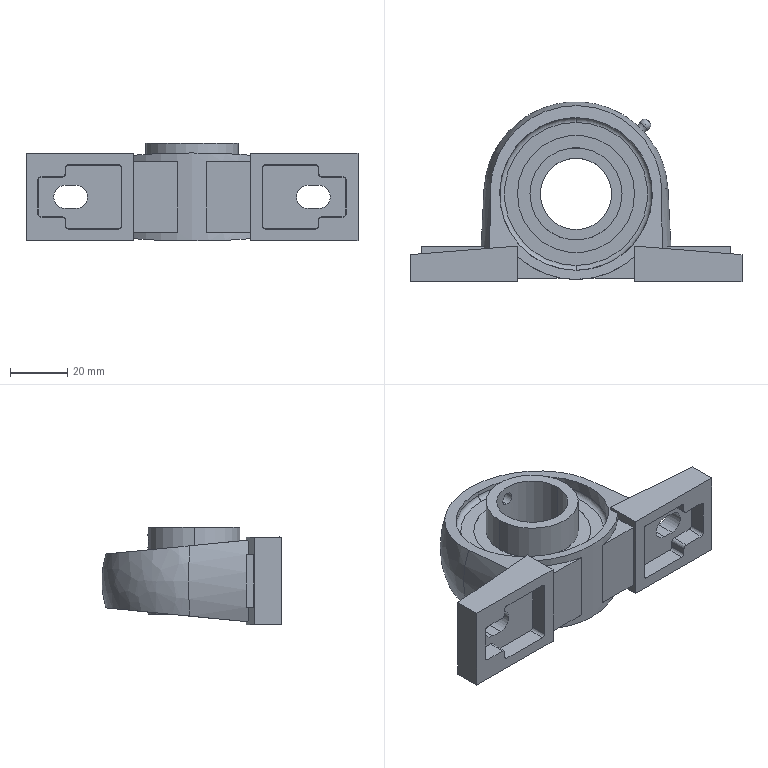Part | SolidWorks | features Revolution 5, Boss 3, Cut 3, RevCut 2, CirPattern 1, Extrusion 1, Scale 1, SweepCut 1 | 1 solid | 123 faces | box 116.25 x 63 x 34.276 mm | volume 65186 mm3 | plane 61 | cylinder 27 | cone 16 | sphere 8 | torus 8 | spline 3 | commonest cylinder face diameters 32.25 x6 41.025 x6 53.452 x6 8.125 x4 4.459 x2 25 x2